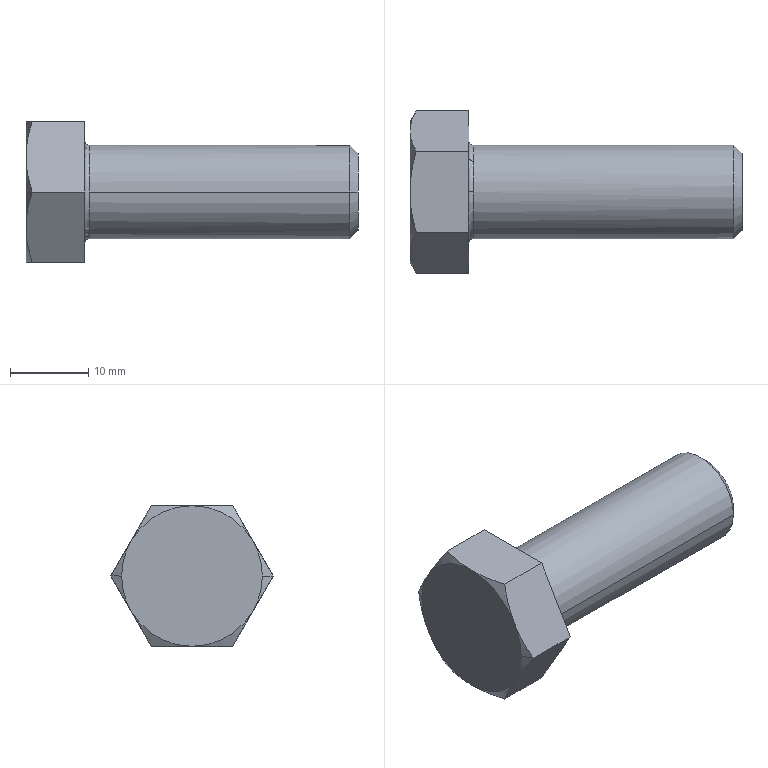Part | STEP file | KS B 1002 - C  M 12 x 35 | 1 solid | 23 faces | box 42.5 x 20.785 x 18 mm | volume 6039 mm3 | cone 10 | plane 9 | torus 2 | cylinder 2 | commonest cylinder face diameters 12 x2